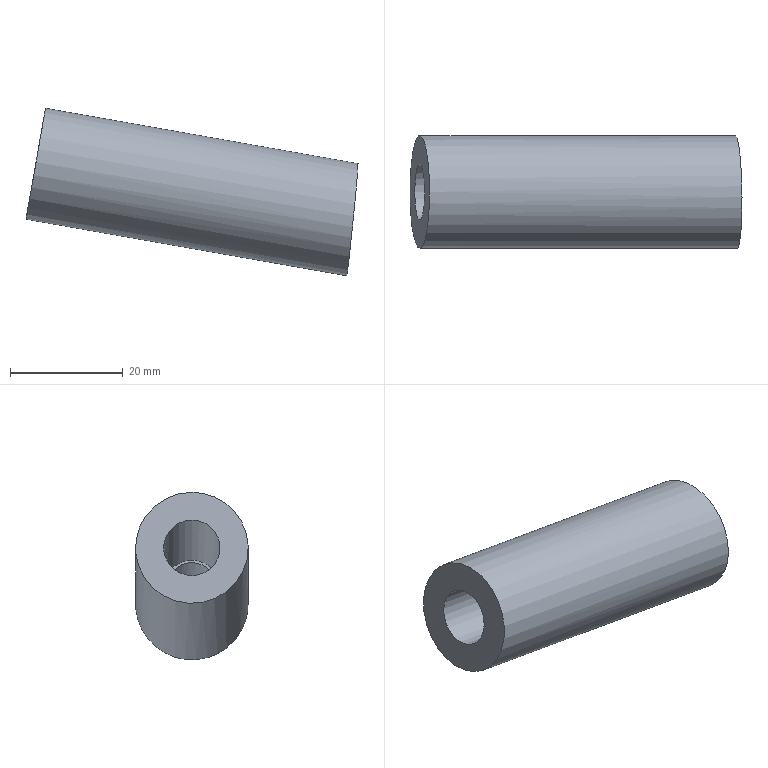Part | NX | features solid 2 | 1 solid | 6 faces | box 58.885 x 20 x 29.723 mm | volume 13644 mm3 | cylinder 3 | plane 2 | spline 1 | commonest cylinder face diameters 9.1 x1 10 x1 20 x1
STEP:
#1=CARTESIAN_POINT('',(-78.297,397.378,-17.241));
#2=VERTEX_POINT('',#1);
#3=CARTESIAN_POINT('',(-80.034,397.378,-27.089));
#4=DIRECTION('',(0.9848,0.,-0.1736));
#5=DIRECTION('',(0.1736,0.,0.9848));
#6=AXIS2_PLACEMENT_3D('',#3,#4,#5);
#7=CIRCLE('',#6,10.);
#8=EDGE_CURVE('',#2,#2,#7,.T.);
#9=ORIENTED_EDGE('',*,*,#8,.F.);
#10=EDGE_LOOP('',(#9));
#11=FACE_BOUND('',#10,.T.);
#12=CARTESIAN_POINT('',(-79.165,397.378,-22.165));
#13=VERTEX_POINT('',#12);
#14=CARTESIAN_POINT('',(-80.034,397.378,-27.089));
#15=DIRECTION('',(0.9848,0.,-0.1736));
#16=DIRECTION('',(0.1736,0.,0.9848));
#17=AXIS2_PLACEMENT_3D('',#14,#15,#16);
#18=CIRCLE('',#17,5.);
#19=EDGE_CURVE('',#13,#13,#18,.F.);
#20=ORIENTED_EDGE('',*,*,#19,.F.);
#21=EDGE_LOOP('',(#20));
#22=FACE_BOUND('',#21,.T.);
#23=CARTESIAN_POINT('',(-80.034,397.378,-27.089));
#24=DIRECTION('',(-0.9848,0.,0.1736));
#25=DIRECTION('',(0.1736,0.,0.9848));
#26=AXIS2_PLACEMENT_3D('',#23,#24,#25);
#27=PLANE('',#26);
#28=ADVANCED_FACE('',(#11,#22),#27,.T.);
#29=ORIENTED_EDGE('',*,*,#8,.T.);
#30=EDGE_LOOP('',(#29));
#31=FACE_BOUND('',#30,.T.);
#32=CARTESIAN_POINT('',(-23.106,390.006,-30.266));
#33=VERTEX_POINT('',#32);
#34=CARTESIAN_POINT('',(-22.782,396.907,-25.935));
#35=CARTESIAN_POINT('',(-23.02,389.204,-29.543));
#36=CARTESIAN_POINT('',(-23.773,386.312,-37.488));
#37=CARTESIAN_POINT('',(-24.597,389.871,-45.142));
#38=CARTESIAN_POINT('',(-25.015,397.852,-48.038));
#39=CARTESIAN_POINT('',(-24.781,405.547,-44.43));
#40=CARTESIAN_POINT('',(-24.034,408.445,-36.499));
#41=CARTESIAN_POINT('',(-23.204,404.89,-28.833));
#42=CARTESIAN_POINT('',(-22.782,396.907,-25.935));
#43=CARTESIAN_POINT('',(-23.02,389.204,-29.543));
#44=CARTESIAN_POINT('',(-23.773,386.312,-37.488));
#45=B_SPLINE_CURVE_WITH_KNOTS('',3,(#34,#35,#36,#37,#38,#39,#40,#41,#42,#43,#44),.UNSPECIFIED.,.T.,.F.,(1,1,1,1,1,1,1,1,1,1,1,1,1,1,1),(-0.02348,-0.01565,-0.007826,0.,0.007826,0.01565,0.02348,0.03131,0.03913,0.04696,0.05478,0.06261,0.07044,0.07826,0.08609),.UNSPECIFIED.);
#46=EDGE_CURVE('',#33,#33,#45,.T.);
#47=ORIENTED_EDGE('',*,*,#46,.F.);
#48=EDGE_LOOP('',(#47));
#49=FACE_BOUND('',#48,.T.);
#50=CARTESIAN_POINT('',(-80.034,397.378,-27.089));
#51=DIRECTION('',(0.9848,0.,-0.1736));
#52=DIRECTION('',(-0.1736,0.,-0.9848));
#53=AXIS2_PLACEMENT_3D('',#50,#51,#52);
#54=CYLINDRICAL_SURFACE('',#53,10.);
#55=ADVANCED_FACE('',(#31,#49),#54,.T.);
#56=CARTESIAN_POINT('',(-23.827,392.828,-36.999));
#57=VERTEX_POINT('',#56);
#58=CARTESIAN_POINT('',(-23.485,393.811,-33.44));
#59=CARTESIAN_POINT('',(-23.819,392.336,-37.001));
#60=CARTESIAN_POINT('',(-24.199,393.811,-40.552));
#61=CARTESIAN_POINT('',(-24.404,397.378,-42.019));
#62=CARTESIAN_POINT('',(-24.313,400.946,-40.531));
#63=CARTESIAN_POINT('',(-23.981,402.418,-36.974));
#64=CARTESIAN_POINT('',(-23.6,400.95,-33.426));
#65=CARTESIAN_POINT('',(-23.394,397.38,-31.954));
#66=CARTESIAN_POINT('',(-23.485,393.811,-33.44));
#67=CARTESIAN_POINT('',(-23.819,392.336,-37.001));
#68=CARTESIAN_POINT('',(-24.199,393.811,-40.552));
#69=B_SPLINE_CURVE_WITH_KNOTS('',3,(#58,#59,#60,#61,#62,#63,#64,#65,#66,#67,#68),.UNSPECIFIED.,.T.,.F.,(1,1,1,1,1,1,1,1,1,1,1,1,1,1,1),(-0.01068,-0.007122,-0.003561,0.,0.003561,0.007122,0.01068,0.01424,0.01781,0.02137,0.02493,0.02849,0.03205,0.03561,0.03917),.UNSPECIFIED.);
#70=EDGE_CURVE('',#57,#57,#69,.T.);
#71=ORIENTED_EDGE('',*,*,#70,.F.);
#72=EDGE_LOOP('',(#71));
#73=FACE_BOUND('',#72,.T.);
#74=ORIENTED_EDGE('',*,*,#46,.T.);
#75=EDGE_LOOP('',(#74));
#76=FACE_BOUND('',#75,.T.);
#77=CARTESIAN_POINT('',(-25.084,407.546,-47.113));
#78=CARTESIAN_POINT('',(-23.048,407.546,-26.828));
#79=CARTESIAN_POINT('',(-25.016,403.478,-47.12));
#80=CARTESIAN_POINT('',(-22.98,403.478,-26.835));
#81=CARTESIAN_POINT('',(-24.949,399.41,-47.127));
#82=CARTESIAN_POINT('',(-22.913,399.41,-26.841));
#83=CARTESIAN_POINT('',(-24.884,395.342,-47.133));
#84=CARTESIAN_POINT('',(-22.848,395.342,-26.848));
#85=CARTESIAN_POINT('',(-24.819,391.274,-47.14));
#86=CARTESIAN_POINT('',(-22.783,391.274,-26.854));
#87=CARTESIAN_POINT('',(-24.756,387.205,-47.146));
#88=CARTESIAN_POINT('',(-22.72,387.205,-26.861));
#89=B_SPLINE_SURFACE_WITH_KNOTS('',5,1,((#77,#78),(#79,#80),(#81,#82),(#83,#84),(#85,#86),(#87,#88)),.SURF_OF_LINEAR_EXTRUSION.,.F.,.F.,.F.,(6,6),(2,2),(0.2405,0.347),(0.4934,0.8012),.PIECEWISE_BEZIER_KNOTS.);
#90=ADVANCED_FACE('',(#73,#76),#89,.F.);
#91=CARTESIAN_POINT('',(-39.657,392.828,-34.208));
#92=VERTEX_POINT('',#91);
#93=CARTESIAN_POINT('',(-39.657,397.378,-34.208));
#94=DIRECTION('',(-0.9848,0.,0.1736));
#95=DIRECTION('',(0.,-1.,0.));
#96=AXIS2_PLACEMENT_3D('',#93,#94,#95);
#97=CIRCLE('',#96,4.55);
#98=EDGE_CURVE('',#92,#92,#97,.T.);
#99=ORIENTED_EDGE('',*,*,#98,.T.);
#100=EDGE_LOOP('',(#99));
#101=FACE_BOUND('',#100,.T.);
#102=ORIENTED_EDGE('',*,*,#70,.T.);
#103=EDGE_LOOP('',(#102));
#104=FACE_BOUND('',#103,.T.);
#105=CARTESIAN_POINT('',(-20.945,397.378,-37.507));
#106=DIRECTION('',(-0.9848,0.,0.1736));
#107=DIRECTION('',(0.,-1.,0.));
#108=AXIS2_PLACEMENT_3D('',#105,#106,#107);
#109=CYLINDRICAL_SURFACE('',#108,4.55);
#110=ADVANCED_FACE('',(#101,#104),#109,.F.);
#111=ORIENTED_EDGE('',*,*,#19,.T.);
#112=EDGE_LOOP('',(#111));
#113=FACE_BOUND('',#112,.T.);
#114=CARTESIAN_POINT('',(-39.657,392.378,-34.208));
#115=VERTEX_POINT('',#114);
#116=CARTESIAN_POINT('',(-39.657,397.378,-34.208));
#117=DIRECTION('',(-0.9848,0.,0.1736));
#118=DIRECTION('',(0.,-1.,0.));
#119=AXIS2_PLACEMENT_3D('',#116,#117,#118);
#120=CIRCLE('',#119,5.);
#121=EDGE_CURVE('',#115,#115,#120,.T.);
#122=ORIENTED_EDGE('',*,*,#121,.F.);
#123=EDGE_LOOP('',(#122));
#124=FACE_BOUND('',#123,.T.);
#125=CARTESIAN_POINT('',(-109.578,397.378,-21.879));
#126=DIRECTION('',(0.9848,0.,-0.1736));
#127=DIRECTION('',(0.,1.,0.));
#128=AXIS2_PLACEMENT_3D('',#125,#126,#127);
#129=CYLINDRICAL_SURFACE('',#128,5.);
#130=ADVANCED_FACE('',(#113,#124),#129,.F.);
#131=ORIENTED_EDGE('',*,*,#98,.F.);
#132=EDGE_LOOP('',(#131));
#133=FACE_BOUND('',#132,.T.);
#134=ORIENTED_EDGE('',*,*,#121,.T.);
#135=EDGE_LOOP('',(#134));
#136=FACE_BOUND('',#135,.T.);
#137=CARTESIAN_POINT('',(-39.657,397.378,-34.208));
#138=DIRECTION('',(-0.9848,0.,0.1736));
#139=DIRECTION('',(0.,-1.,0.));
#140=AXIS2_PLACEMENT_3D('',#137,#138,#139);
#141=PLANE('',#140);
#142=ADVANCED_FACE('',(#133,#136),#141,.T.);
#143=CLOSED_SHELL('',(#28,#55,#90,#110,#130,#142));
#144=MANIFOLD_SOLID_BREP('',#143);
#145=(LENGTH_UNIT()NAMED_UNIT(*)SI_UNIT(.MILLI.,.METRE.));
#146=UNCERTAINTY_MEASURE_WITH_UNIT(LENGTH_MEASURE(0.0508),#145,'','');
#147=(NAMED_UNIT(*)PLANE_ANGLE_UNIT()SI_UNIT($,.RADIAN.));
#148=(NAMED_UNIT(*)SI_UNIT($,.STERADIAN.)SOLID_ANGLE_UNIT());
#149=(GEOMETRIC_REPRESENTATION_CONTEXT(3)GLOBAL_UNCERTAINTY_ASSIGNED_CONTEXT((#146))GLOBAL_UNIT_ASSIGNED_CONTEXT((#145,#147,#148))REPRESENTATION_CONTEXT('',''));
#150=ADVANCED_BREP_SHAPE_REPRESENTATION('',(#144),#149);